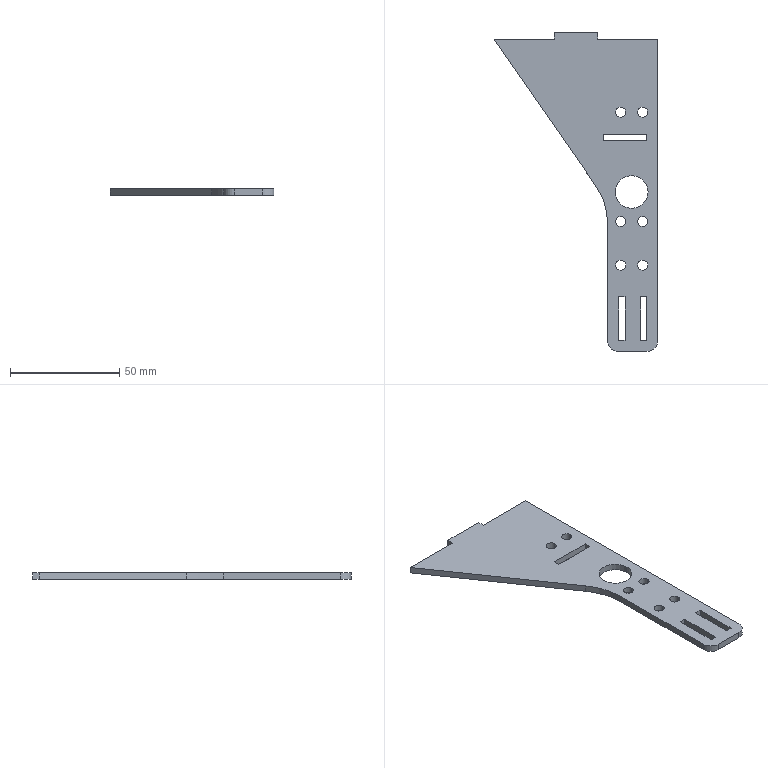Part | SolidWorks | features Cut 3, Fillet 2, Extrusion 1 | 1 solid | 40 faces | box 75 x 146 x 3 mm | volume 14540 mm3 | plane 23 | cylinder 17 | commonest cylinder face diameters 4.6 x12 10 x2 15 x2 60 x1
STEP:
#1=CARTESIAN_POINT('',(-9.25,39.5,0.));
#2=VERTEX_POINT('',#1);
#3=CARTESIAN_POINT('',(-4.65,39.5,0.));
#4=VERTEX_POINT('',#3);
#5=CARTESIAN_POINT('',(-6.95,39.5,0.));
#6=DIRECTION('',(0.,0.,1.));
#7=DIRECTION('',(1.,0.,0.));
#8=AXIS2_PLACEMENT_3D('',#5,#6,#7);
#9=CIRCLE('',#8,2.3);
#10=EDGE_CURVE('',#2,#4,#9,.T.);
#11=ORIENTED_EDGE('',*,*,#10,.F.);
#12=CARTESIAN_POINT('',(-9.25,39.5,3.));
#13=VERTEX_POINT('',#12);
#14=CARTESIAN_POINT('',(-9.25,39.5,0.));
#15=DIRECTION('',(0.,0.,1.));
#16=VECTOR('',#15,1000.);
#17=LINE('',#14,#16);
#18=EDGE_CURVE('',#2,#13,#17,.T.);
#19=ORIENTED_EDGE('',*,*,#18,.T.);
#20=CARTESIAN_POINT('',(-4.65,39.5,3.));
#21=VERTEX_POINT('',#20);
#22=CARTESIAN_POINT('',(-6.95,39.5,3.));
#23=DIRECTION('',(0.,0.,1.));
#24=DIRECTION('',(1.,0.,0.));
#25=AXIS2_PLACEMENT_3D('',#22,#23,#24);
#26=CIRCLE('',#25,2.3);
#27=EDGE_CURVE('',#13,#21,#26,.T.);
#28=ORIENTED_EDGE('',*,*,#27,.T.);
#29=CARTESIAN_POINT('',(-4.65,39.5,0.));
#30=DIRECTION('',(0.,0.,1.));
#31=VECTOR('',#30,1000.);
#32=LINE('',#29,#31);
#33=EDGE_CURVE('',#4,#21,#32,.T.);
#34=ORIENTED_EDGE('',*,*,#33,.F.);
#35=EDGE_LOOP('',(#11,#19,#28,#34));
#36=FACE_OUTER_BOUND('',#35,.T.);
#37=CARTESIAN_POINT('',(-6.95,39.5,0.));
#38=DIRECTION('',(0.,0.,1.));
#39=DIRECTION('',(1.,0.,0.));
#40=AXIS2_PLACEMENT_3D('',#37,#38,#39);
#41=CYLINDRICAL_SURFACE('',#40,2.3);
#42=ADVANCED_FACE('',(#36),#41,.F.);
#43=CARTESIAN_POINT('',(-19.35,39.5,0.));
#44=VERTEX_POINT('',#43);
#45=CARTESIAN_POINT('',(-14.75,39.5,0.));
#46=VERTEX_POINT('',#45);
#47=CARTESIAN_POINT('',(-17.05,39.5,0.));
#48=DIRECTION('',(0.,0.,1.));
#49=DIRECTION('',(1.,0.,0.));
#50=AXIS2_PLACEMENT_3D('',#47,#48,#49);
#51=CIRCLE('',#50,2.3);
#52=EDGE_CURVE('',#44,#46,#51,.T.);
#53=ORIENTED_EDGE('',*,*,#52,.F.);
#54=CARTESIAN_POINT('',(-19.35,39.5,3.));
#55=VERTEX_POINT('',#54);
#56=CARTESIAN_POINT('',(-19.35,39.5,0.));
#57=DIRECTION('',(0.,0.,1.));
#58=VECTOR('',#57,1000.);
#59=LINE('',#56,#58);
#60=EDGE_CURVE('',#44,#55,#59,.T.);
#61=ORIENTED_EDGE('',*,*,#60,.T.);
#62=CARTESIAN_POINT('',(-14.75,39.5,3.));
#63=VERTEX_POINT('',#62);
#64=CARTESIAN_POINT('',(-17.05,39.5,3.));
#65=DIRECTION('',(0.,0.,1.));
#66=DIRECTION('',(1.,0.,0.));
#67=AXIS2_PLACEMENT_3D('',#64,#65,#66);
#68=CIRCLE('',#67,2.3);
#69=EDGE_CURVE('',#55,#63,#68,.T.);
#70=ORIENTED_EDGE('',*,*,#69,.T.);
#71=CARTESIAN_POINT('',(-14.75,39.5,0.));
#72=DIRECTION('',(0.,0.,1.));
#73=VECTOR('',#72,1000.);
#74=LINE('',#71,#73);
#75=EDGE_CURVE('',#46,#63,#74,.T.);
#76=ORIENTED_EDGE('',*,*,#75,.F.);
#77=EDGE_LOOP('',(#53,#61,#70,#76));
#78=FACE_OUTER_BOUND('',#77,.T.);
#79=CARTESIAN_POINT('',(-17.05,39.5,0.));
#80=DIRECTION('',(0.,0.,1.));
#81=DIRECTION('',(1.,0.,0.));
#82=AXIS2_PLACEMENT_3D('',#79,#80,#81);
#83=CYLINDRICAL_SURFACE('',#82,2.3);
#84=ADVANCED_FACE('',(#78),#83,.F.);
#85=CARTESIAN_POINT('',(-4.65,109.5,3.));
#86=VERTEX_POINT('',#85);
#87=CARTESIAN_POINT('',(-9.25,109.5,3.));
#88=VERTEX_POINT('',#87);
#89=CARTESIAN_POINT('',(-6.95,109.5,3.));
#90=DIRECTION('',(0.,0.,-1.));
#91=DIRECTION('',(1.,0.,0.));
#92=AXIS2_PLACEMENT_3D('',#89,#90,#91);
#93=CIRCLE('',#92,2.3);
#94=EDGE_CURVE('',#86,#88,#93,.T.);
#95=ORIENTED_EDGE('',*,*,#94,.F.);
#96=CARTESIAN_POINT('',(-4.65,109.5,0.));
#97=VERTEX_POINT('',#96);
#98=CARTESIAN_POINT('',(-4.65,109.5,3.001));
#99=DIRECTION('',(0.,0.,-1.));
#100=VECTOR('',#99,1000.);
#101=LINE('',#98,#100);
#102=EDGE_CURVE('',#86,#97,#101,.T.);
#103=ORIENTED_EDGE('',*,*,#102,.T.);
#104=CARTESIAN_POINT('',(-9.25,109.5,0.));
#105=VERTEX_POINT('',#104);
#106=CARTESIAN_POINT('',(-6.95,109.5,0.));
#107=DIRECTION('',(0.,0.,-1.));
#108=DIRECTION('',(-1.,0.,0.));
#109=AXIS2_PLACEMENT_3D('',#106,#107,#108);
#110=CIRCLE('',#109,2.3);
#111=EDGE_CURVE('',#97,#105,#110,.T.);
#112=ORIENTED_EDGE('',*,*,#111,.T.);
#113=CARTESIAN_POINT('',(-9.25,109.5,3.001));
#114=DIRECTION('',(0.,0.,-1.));
#115=VECTOR('',#114,1000.);
#116=LINE('',#113,#115);
#117=EDGE_CURVE('',#88,#105,#116,.T.);
#118=ORIENTED_EDGE('',*,*,#117,.F.);
#119=EDGE_LOOP('',(#95,#103,#112,#118));
#120=FACE_OUTER_BOUND('',#119,.T.);
#121=CARTESIAN_POINT('',(-6.95,109.5,3.001));
#122=DIRECTION('',(0.,0.,-1.));
#123=DIRECTION('',(-1.,0.,0.));
#124=AXIS2_PLACEMENT_3D('',#121,#122,#123);
#125=CYLINDRICAL_SURFACE('',#124,2.3);
#126=ADVANCED_FACE('',(#120),#125,.F.);
#127=CARTESIAN_POINT('',(-14.75,109.5,3.));
#128=VERTEX_POINT('',#127);
#129=CARTESIAN_POINT('',(-19.35,109.5,3.));
#130=VERTEX_POINT('',#129);
#131=CARTESIAN_POINT('',(-17.05,109.5,3.));
#132=DIRECTION('',(0.,0.,-1.));
#133=DIRECTION('',(1.,0.,0.));
#134=AXIS2_PLACEMENT_3D('',#131,#132,#133);
#135=CIRCLE('',#134,2.3);
#136=EDGE_CURVE('',#128,#130,#135,.T.);
#137=ORIENTED_EDGE('',*,*,#136,.F.);
#138=CARTESIAN_POINT('',(-14.75,109.5,0.));
#139=VERTEX_POINT('',#138);
#140=CARTESIAN_POINT('',(-14.75,109.5,3.001));
#141=DIRECTION('',(0.,0.,-1.));
#142=VECTOR('',#141,1000.);
#143=LINE('',#140,#142);
#144=EDGE_CURVE('',#128,#139,#143,.T.);
#145=ORIENTED_EDGE('',*,*,#144,.T.);
#146=CARTESIAN_POINT('',(-19.35,109.5,0.));
#147=VERTEX_POINT('',#146);
#148=CARTESIAN_POINT('',(-17.05,109.5,0.));
#149=DIRECTION('',(0.,0.,-1.));
#150=DIRECTION('',(-1.,0.,0.));
#151=AXIS2_PLACEMENT_3D('',#148,#149,#150);
#152=CIRCLE('',#151,2.3);
#153=EDGE_CURVE('',#139,#147,#152,.T.);
#154=ORIENTED_EDGE('',*,*,#153,.T.);
#155=CARTESIAN_POINT('',(-19.35,109.5,3.001));
#156=DIRECTION('',(0.,0.,-1.));
#157=VECTOR('',#156,1000.);
#158=LINE('',#155,#157);
#159=EDGE_CURVE('',#130,#147,#158,.T.);
#160=ORIENTED_EDGE('',*,*,#159,.F.);
#161=EDGE_LOOP('',(#137,#145,#154,#160));
#162=FACE_OUTER_BOUND('',#161,.T.);
#163=CARTESIAN_POINT('',(-17.05,109.5,3.001));
#164=DIRECTION('',(0.,0.,-1.));
#165=DIRECTION('',(-1.,0.,0.));
#166=AXIS2_PLACEMENT_3D('',#163,#164,#165);
#167=CYLINDRICAL_SURFACE('',#166,2.3);
#168=ADVANCED_FACE('',(#162),#167,.F.);
#169=CARTESIAN_POINT('',(-4.65,59.5,3.));
#170=VERTEX_POINT('',#169);
#171=CARTESIAN_POINT('',(-9.25,59.5,3.));
#172=VERTEX_POINT('',#171);
#173=CARTESIAN_POINT('',(-6.95,59.5,3.));
#174=DIRECTION('',(0.,0.,-1.));
#175=DIRECTION('',(1.,0.,0.));
#176=AXIS2_PLACEMENT_3D('',#173,#174,#175);
#177=CIRCLE('',#176,2.3);
#178=EDGE_CURVE('',#170,#172,#177,.T.);
#179=ORIENTED_EDGE('',*,*,#178,.F.);
#180=CARTESIAN_POINT('',(-4.65,59.5,0.));
#181=VERTEX_POINT('',#180);
#182=CARTESIAN_POINT('',(-4.65,59.5,3.001));
#183=DIRECTION('',(0.,0.,-1.));
#184=VECTOR('',#183,1000.);
#185=LINE('',#182,#184);
#186=EDGE_CURVE('',#170,#181,#185,.T.);
#187=ORIENTED_EDGE('',*,*,#186,.T.);
#188=CARTESIAN_POINT('',(-9.25,59.5,0.));
#189=VERTEX_POINT('',#188);
#190=CARTESIAN_POINT('',(-6.95,59.5,0.));
#191=DIRECTION('',(0.,0.,-1.));
#192=DIRECTION('',(-1.,0.,0.));
#193=AXIS2_PLACEMENT_3D('',#190,#191,#192);
#194=CIRCLE('',#193,2.3);
#195=EDGE_CURVE('',#181,#189,#194,.T.);
#196=ORIENTED_EDGE('',*,*,#195,.T.);
#197=CARTESIAN_POINT('',(-9.25,59.5,3.001));
#198=DIRECTION('',(0.,0.,-1.));
#199=VECTOR('',#198,1000.);
#200=LINE('',#197,#199);
#201=EDGE_CURVE('',#172,#189,#200,.T.);
#202=ORIENTED_EDGE('',*,*,#201,.F.);
#203=EDGE_LOOP('',(#179,#187,#196,#202));
#204=FACE_OUTER_BOUND('',#203,.T.);
#205=CARTESIAN_POINT('',(-6.95,59.5,3.001));
#206=DIRECTION('',(0.,0.,-1.));
#207=DIRECTION('',(-1.,0.,0.));
#208=AXIS2_PLACEMENT_3D('',#205,#206,#207);
#209=CYLINDRICAL_SURFACE('',#208,2.3);
#210=ADVANCED_FACE('',(#204),#209,.F.);
#211=CARTESIAN_POINT('',(-14.75,59.5,3.));
#212=VERTEX_POINT('',#211);
#213=CARTESIAN_POINT('',(-19.35,59.5,3.));
#214=VERTEX_POINT('',#213);
#215=CARTESIAN_POINT('',(-17.05,59.5,3.));
#216=DIRECTION('',(0.,0.,-1.));
#217=DIRECTION('',(1.,0.,0.));
#218=AXIS2_PLACEMENT_3D('',#215,#216,#217);
#219=CIRCLE('',#218,2.3);
#220=EDGE_CURVE('',#212,#214,#219,.T.);
#221=ORIENTED_EDGE('',*,*,#220,.F.);
#222=CARTESIAN_POINT('',(-14.75,59.5,0.));
#223=VERTEX_POINT('',#222);
#224=CARTESIAN_POINT('',(-14.75,59.5,3.001));
#225=DIRECTION('',(0.,0.,-1.));
#226=VECTOR('',#225,1000.);
#227=LINE('',#224,#226);
#228=EDGE_CURVE('',#212,#223,#227,.T.);
#229=ORIENTED_EDGE('',*,*,#228,.T.);
#230=CARTESIAN_POINT('',(-19.35,59.5,0.));
#231=VERTEX_POINT('',#230);
#232=CARTESIAN_POINT('',(-17.05,59.5,0.));
#233=DIRECTION('',(0.,0.,-1.));
#234=DIRECTION('',(-1.,0.,0.));
#235=AXIS2_PLACEMENT_3D('',#232,#233,#234);
#236=CIRCLE('',#235,2.3);
#237=EDGE_CURVE('',#223,#231,#236,.T.);
#238=ORIENTED_EDGE('',*,*,#237,.T.);
#239=CARTESIAN_POINT('',(-19.35,59.5,3.001));
#240=DIRECTION('',(0.,0.,-1.));
#241=VECTOR('',#240,1000.);
#242=LINE('',#239,#241);
#243=EDGE_CURVE('',#214,#231,#242,.T.);
#244=ORIENTED_EDGE('',*,*,#243,.F.);
#245=EDGE_LOOP('',(#221,#229,#238,#244));
#246=FACE_OUTER_BOUND('',#245,.T.);
#247=CARTESIAN_POINT('',(-17.05,59.5,3.001));
#248=DIRECTION('',(0.,0.,-1.));
#249=DIRECTION('',(-1.,0.,0.));
#250=AXIS2_PLACEMENT_3D('',#247,#248,#249);
#251=CYLINDRICAL_SURFACE('',#250,2.3);
#252=ADVANCED_FACE('',(#246),#251,.F.);
#253=CARTESIAN_POINT('',(-4.5,73.,3.));
#254=VERTEX_POINT('',#253);
#255=CARTESIAN_POINT('',(-19.5,73.,3.));
#256=VERTEX_POINT('',#255);
#257=CARTESIAN_POINT('',(-12.,73.,3.));
#258=DIRECTION('',(0.,0.,-1.));
#259=DIRECTION('',(1.,0.,0.));
#260=AXIS2_PLACEMENT_3D('',#257,#258,#259);
#261=CIRCLE('',#260,7.5);
#262=EDGE_CURVE('',#254,#256,#261,.T.);
#263=ORIENTED_EDGE('',*,*,#262,.F.);
#264=CARTESIAN_POINT('',(-4.5,73.,0.));
#265=VERTEX_POINT('',#264);
#266=CARTESIAN_POINT('',(-4.5,73.,3.001));
#267=DIRECTION('',(0.,0.,-1.));
#268=VECTOR('',#267,1000.);
#269=LINE('',#266,#268);
#270=EDGE_CURVE('',#254,#265,#269,.T.);
#271=ORIENTED_EDGE('',*,*,#270,.T.);
#272=CARTESIAN_POINT('',(-19.5,73.,0.));
#273=VERTEX_POINT('',#272);
#274=CARTESIAN_POINT('',(-12.,73.,0.));
#275=DIRECTION('',(0.,0.,-1.));
#276=DIRECTION('',(-1.,0.,0.));
#277=AXIS2_PLACEMENT_3D('',#274,#275,#276);
#278=CIRCLE('',#277,7.5);
#279=EDGE_CURVE('',#265,#273,#278,.T.);
#280=ORIENTED_EDGE('',*,*,#279,.T.);
#281=CARTESIAN_POINT('',(-19.5,73.,3.001));
#282=DIRECTION('',(0.,0.,-1.));
#283=VECTOR('',#282,1000.);
#284=LINE('',#281,#283);
#285=EDGE_CURVE('',#256,#273,#284,.T.);
#286=ORIENTED_EDGE('',*,*,#285,.F.);
#287=EDGE_LOOP('',(#263,#271,#280,#286));
#288=FACE_OUTER_BOUND('',#287,.T.);
#289=CARTESIAN_POINT('',(-12.,73.,3.001));
#290=DIRECTION('',(0.,0.,-1.));
#291=DIRECTION('',(-1.,0.,0.));
#292=AXIS2_PLACEMENT_3D('',#289,#290,#291);
#293=CYLINDRICAL_SURFACE('',#292,7.5);
#294=ADVANCED_FACE('',(#288),#293,.F.);
#295=CARTESIAN_POINT('',(-6.95,39.5,3.));
#296=DIRECTION('',(0.,0.,1.));
#297=DIRECTION('',(1.,0.,0.));
#298=AXIS2_PLACEMENT_3D('',#295,#296,#297);
#299=CIRCLE('',#298,2.3);
#300=EDGE_CURVE('',#21,#13,#299,.T.);
#301=ORIENTED_EDGE('',*,*,#300,.F.);
#302=ORIENTED_EDGE('',*,*,#27,.F.);
#303=EDGE_LOOP('',(#301,#302));
#304=FACE_BOUND('',#303,.T.);
#305=CARTESIAN_POINT('',(-17.05,39.5,3.));
#306=DIRECTION('',(0.,0.,1.));
#307=DIRECTION('',(1.,0.,0.));
#308=AXIS2_PLACEMENT_3D('',#305,#306,#307);
#309=CIRCLE('',#308,2.3);
#310=EDGE_CURVE('',#63,#55,#309,.T.);
#311=ORIENTED_EDGE('',*,*,#310,.F.);
#312=ORIENTED_EDGE('',*,*,#69,.F.);
#313=EDGE_LOOP('',(#311,#312));
#314=FACE_BOUND('',#313,.T.);
#315=CARTESIAN_POINT('',(-5.,96.55,3.));
#316=VERTEX_POINT('',#315);
#317=CARTESIAN_POINT('',(-25.,96.55,3.));
#318=VERTEX_POINT('',#317);
#319=CARTESIAN_POINT('',(-5.,96.55,3.));
#320=DIRECTION('',(-1.,0.,0.));
#321=VECTOR('',#320,1000.);
#322=LINE('',#319,#321);
#323=EDGE_CURVE('',#316,#318,#322,.T.);
#324=ORIENTED_EDGE('',*,*,#323,.T.);
#325=CARTESIAN_POINT('',(-25.,99.45,3.));
#326=VERTEX_POINT('',#325);
#327=CARTESIAN_POINT('',(-25.,96.55,3.));
#328=DIRECTION('',(0.,1.,0.));
#329=VECTOR('',#328,1000.);
#330=LINE('',#327,#329);
#331=EDGE_CURVE('',#318,#326,#330,.T.);
#332=ORIENTED_EDGE('',*,*,#331,.T.);
#333=CARTESIAN_POINT('',(-5.,99.45,3.));
#334=VERTEX_POINT('',#333);
#335=CARTESIAN_POINT('',(-25.,99.45,3.));
#336=DIRECTION('',(1.,0.,0.));
#337=VECTOR('',#336,1000.);
#338=LINE('',#335,#337);
#339=EDGE_CURVE('',#326,#334,#338,.T.);
#340=ORIENTED_EDGE('',*,*,#339,.T.);
#341=CARTESIAN_POINT('',(-5.,99.45,3.));
#342=DIRECTION('',(0.,-1.,0.));
#343=VECTOR('',#342,1000.);
#344=LINE('',#341,#343);
#345=EDGE_CURVE('',#334,#316,#344,.T.);
#346=ORIENTED_EDGE('',*,*,#345,.T.);
#347=EDGE_LOOP('',(#324,#332,#340,#346));
#348=FACE_BOUND('',#347,.T.);
#349=CARTESIAN_POINT('',(-6.95,109.5,3.));
#350=DIRECTION('',(0.,0.,-1.));
#351=DIRECTION('',(1.,0.,0.));
#352=AXIS2_PLACEMENT_3D('',#349,#350,#351);
#353=CIRCLE('',#352,2.3);
#354=EDGE_CURVE('',#88,#86,#353,.T.);
#355=ORIENTED_EDGE('',*,*,#354,.T.);
#356=ORIENTED_EDGE('',*,*,#94,.T.);
#357=EDGE_LOOP('',(#355,#356));
#358=FACE_BOUND('',#357,.T.);
#359=CARTESIAN_POINT('',(-17.05,109.5,3.));
#360=DIRECTION('',(0.,0.,-1.));
#361=DIRECTION('',(1.,0.,0.));
#362=AXIS2_PLACEMENT_3D('',#359,#360,#361);
#363=CIRCLE('',#362,2.3);
#364=EDGE_CURVE('',#130,#128,#363,.T.);
#365=ORIENTED_EDGE('',*,*,#364,.T.);
#366=ORIENTED_EDGE('',*,*,#136,.T.);
#367=EDGE_LOOP('',(#365,#366));
#368=FACE_BOUND('',#367,.T.);
#369=CARTESIAN_POINT('',(-6.95,59.5,3.));
#370=DIRECTION('',(0.,0.,-1.));
#371=DIRECTION('',(1.,0.,0.));
#372=AXIS2_PLACEMENT_3D('',#369,#370,#371);
#373=CIRCLE('',#372,2.3);
#374=EDGE_CURVE('',#172,#170,#373,.T.);
#375=ORIENTED_EDGE('',*,*,#374,.T.);
#376=ORIENTED_EDGE('',*,*,#178,.T.);
#377=EDGE_LOOP('',(#375,#376));
#378=FACE_BOUND('',#377,.T.);
#379=CARTESIAN_POINT('',(-17.05,59.5,3.));
#380=DIRECTION('',(0.,0.,-1.));
#381=DIRECTION('',(1.,0.,0.));
#382=AXIS2_PLACEMENT_3D('',#379,#380,#381);
#383=CIRCLE('',#382,2.3);
#384=EDGE_CURVE('',#214,#212,#383,.T.);
#385=ORIENTED_EDGE('',*,*,#384,.T.);
#386=ORIENTED_EDGE('',*,*,#220,.T.);
#387=EDGE_LOOP('',(#385,#386));
#388=FACE_BOUND('',#387,.T.);
#389=CARTESIAN_POINT('',(-12.,73.,3.));
#390=DIRECTION('',(0.,0.,-1.));
#391=DIRECTION('',(1.,0.,0.));
#392=AXIS2_PLACEMENT_3D('',#389,#390,#391);
#393=CIRCLE('',#392,7.5);
#394=EDGE_CURVE('',#256,#254,#393,.T.);
#395=ORIENTED_EDGE('',*,*,#394,.T.);
#396=ORIENTED_EDGE('',*,*,#262,.T.);
#397=EDGE_LOOP('',(#395,#396));
#398=FACE_BOUND('',#397,.T.);
#399=CARTESIAN_POINT('',(-17.95,5.,3.));
#400=VERTEX_POINT('',#399);
#401=CARTESIAN_POINT('',(-15.05,5.,3.));
#402=VERTEX_POINT('',#401);
#403=CARTESIAN_POINT('',(-17.95,5.,3.));
#404=DIRECTION('',(1.,0.,0.));
#405=VECTOR('',#404,1000.);
#406=LINE('',#403,#405);
#407=EDGE_CURVE('',#400,#402,#406,.T.);
#408=ORIENTED_EDGE('',*,*,#407,.F.);
#409=CARTESIAN_POINT('',(-17.95,25.,3.));
#410=VERTEX_POINT('',#409);
#411=CARTESIAN_POINT('',(-17.95,25.,3.));
#412=DIRECTION('',(0.,-1.,0.));
#413=VECTOR('',#412,1000.);
#414=LINE('',#411,#413);
#415=EDGE_CURVE('',#410,#400,#414,.T.);
#416=ORIENTED_EDGE('',*,*,#415,.F.);
#417=CARTESIAN_POINT('',(-15.05,25.,3.));
#418=VERTEX_POINT('',#417);
#419=CARTESIAN_POINT('',(-17.95,25.,3.));
#420=DIRECTION('',(-1.,0.,0.));
#421=VECTOR('',#420,1000.);
#422=LINE('',#419,#421);
#423=EDGE_CURVE('',#418,#410,#422,.T.);
#424=ORIENTED_EDGE('',*,*,#423,.F.);
#425=CARTESIAN_POINT('',(-15.05,25.,3.));
#426=DIRECTION('',(0.,1.,0.));
#427=VECTOR('',#426,1000.);
#428=LINE('',#425,#427);
#429=EDGE_CURVE('',#402,#418,#428,.T.);
#430=ORIENTED_EDGE('',*,*,#429,.F.);
#431=EDGE_LOOP('',(#408,#416,#424,#430));
#432=FACE_BOUND('',#431,.T.);
#433=CARTESIAN_POINT('',(-18.,0.,3.));
#434=VERTEX_POINT('',#433);
#435=CARTESIAN_POINT('',(-5.,0.,3.));
#436=VERTEX_POINT('',#435);
#437=CARTESIAN_POINT('',(0.,0.,3.));
#438=DIRECTION('',(1.,0.,0.));
#439=VECTOR('',#438,1000.);
#440=LINE('',#437,#439);
#441=EDGE_CURVE('',#434,#436,#440,.T.);
#442=ORIENTED_EDGE('',*,*,#441,.T.);
#443=CARTESIAN_POINT('',(0.,5.,3.));
#444=VERTEX_POINT('',#443);
#445=CARTESIAN_POINT('',(-5.,5.,3.));
#446=DIRECTION('',(0.,0.,1.));
#447=DIRECTION('',(1.,0.,0.));
#448=AXIS2_PLACEMENT_3D('',#445,#446,#447);
#449=CIRCLE('',#448,5.);
#450=EDGE_CURVE('',#436,#444,#449,.T.);
#451=ORIENTED_EDGE('',*,*,#450,.T.);
#452=CARTESIAN_POINT('',(0.,143.,3.));
#453=VERTEX_POINT('',#452);
#454=CARTESIAN_POINT('',(0.,0.,3.));
#455=DIRECTION('',(0.,1.,0.));
#456=VECTOR('',#455,1000.);
#457=LINE('',#454,#456);
#458=EDGE_CURVE('',#444,#453,#457,.T.);
#459=ORIENTED_EDGE('',*,*,#458,.T.);
#460=CARTESIAN_POINT('',(-27.5,143.,3.));
#461=VERTEX_POINT('',#460);
#462=CARTESIAN_POINT('',(0.,143.,3.));
#463=DIRECTION('',(-1.,0.,0.));
#464=VECTOR('',#463,1000.);
#465=LINE('',#462,#464);
#466=EDGE_CURVE('',#453,#461,#465,.T.);
#467=ORIENTED_EDGE('',*,*,#466,.T.);
#468=CARTESIAN_POINT('',(-27.5,146.,3.));
#469=VERTEX_POINT('',#468);
#470=CARTESIAN_POINT('',(-27.5,143.,3.));
#471=DIRECTION('',(0.,1.,0.));
#472=VECTOR('',#471,1000.);
#473=LINE('',#470,#472);
#474=EDGE_CURVE('',#461,#469,#473,.T.);
#475=ORIENTED_EDGE('',*,*,#474,.T.);
#476=CARTESIAN_POINT('',(-47.5,146.,3.));
#477=VERTEX_POINT('',#476);
#478=CARTESIAN_POINT('',(-47.5,146.,3.));
#479=DIRECTION('',(-1.,0.,0.));
#480=VECTOR('',#479,1000.);
#481=LINE('',#478,#480);
#482=EDGE_CURVE('',#469,#477,#481,.T.);
#483=ORIENTED_EDGE('',*,*,#482,.T.);
#484=CARTESIAN_POINT('',(-47.5,143.,3.));
#485=VERTEX_POINT('',#484);
#486=CARTESIAN_POINT('',(-47.5,143.,3.));
#487=DIRECTION('',(0.,-1.,0.));
#488=VECTOR('',#487,1000.);
#489=LINE('',#486,#488);
#490=EDGE_CURVE('',#477,#485,#489,.T.);
#491=ORIENTED_EDGE('',*,*,#490,.T.);
#492=CARTESIAN_POINT('',(-75.,143.,3.));
#493=VERTEX_POINT('',#492);
#494=CARTESIAN_POINT('',(-75.,143.,3.));
#495=DIRECTION('',(-1.,0.,0.));
#496=VECTOR('',#495,1000.);
#497=LINE('',#494,#496);
#498=EDGE_CURVE('',#485,#493,#497,.T.);
#499=ORIENTED_EDGE('',*,*,#498,.T.);
#500=CARTESIAN_POINT('',(-28.346,75.711,3.));
#501=VERTEX_POINT('',#500);
#502=CARTESIAN_POINT('',(-23.,68.,3.));
#503=DIRECTION('',(0.5698,-0.8218,0.));
#504=VECTOR('',#503,1000.);
#505=LINE('',#502,#504);
#506=EDGE_CURVE('',#493,#501,#505,.T.);
#507=ORIENTED_EDGE('',*,*,#506,.T.);
#508=CARTESIAN_POINT('',(-23.,58.617,3.));
#509=VERTEX_POINT('',#508);
#510=CARTESIAN_POINT('',(-53.,58.617,3.));
#511=DIRECTION('',(0.,0.,-1.));
#512=DIRECTION('',(1.,0.,0.));
#513=AXIS2_PLACEMENT_3D('',#510,#511,#512);
#514=CIRCLE('',#513,30.);
#515=EDGE_CURVE('',#501,#509,#514,.T.);
#516=ORIENTED_EDGE('',*,*,#515,.T.);
#517=CARTESIAN_POINT('',(-23.,5.,3.));
#518=VERTEX_POINT('',#517);
#519=CARTESIAN_POINT('',(-23.,0.,3.));
#520=DIRECTION('',(0.,-1.,0.));
#521=VECTOR('',#520,1000.);
#522=LINE('',#519,#521);
#523=EDGE_CURVE('',#509,#518,#522,.T.);
#524=ORIENTED_EDGE('',*,*,#523,.T.);
#525=CARTESIAN_POINT('',(-18.,5.,3.));
#526=DIRECTION('',(0.,0.,1.));
#527=DIRECTION('',(1.,0.,0.));
#528=AXIS2_PLACEMENT_3D('',#525,#526,#527);
#529=CIRCLE('',#528,5.);
#530=EDGE_CURVE('',#518,#434,#529,.T.);
#531=ORIENTED_EDGE('',*,*,#530,.T.);
#532=EDGE_LOOP('',(#442,#451,#459,#467,#475,#483,#491,#499,#507,#516,#524,#531));
#533=FACE_OUTER_BOUND('',#532,.T.);
#534=CARTESIAN_POINT('',(-7.95,5.,3.));
#535=VERTEX_POINT('',#534);
#536=CARTESIAN_POINT('',(-5.05,5.,3.));
#537=VERTEX_POINT('',#536);
#538=CARTESIAN_POINT('',(-7.95,5.,3.));
#539=DIRECTION('',(1.,0.,0.));
#540=VECTOR('',#539,1000.);
#541=LINE('',#538,#540);
#542=EDGE_CURVE('',#535,#537,#541,.T.);
#543=ORIENTED_EDGE('',*,*,#542,.F.);
#544=CARTESIAN_POINT('',(-7.95,25.,3.));
#545=VERTEX_POINT('',#544);
#546=CARTESIAN_POINT('',(-7.95,5.,3.));
#547=DIRECTION('',(0.,-1.,0.));
#548=VECTOR('',#547,1000.);
#549=LINE('',#546,#548);
#550=EDGE_CURVE('',#545,#535,#549,.T.);
#551=ORIENTED_EDGE('',*,*,#550,.F.);
#552=CARTESIAN_POINT('',(-5.05,25.,3.));
#553=VERTEX_POINT('',#552);
#554=CARTESIAN_POINT('',(-7.95,25.,3.));
#555=DIRECTION('',(-1.,0.,0.));
#556=VECTOR('',#555,1000.);
#557=LINE('',#554,#556);
#558=EDGE_CURVE('',#553,#545,#557,.T.);
#559=ORIENTED_EDGE('',*,*,#558,.F.);
#560=CARTESIAN_POINT('',(-5.05,5.,3.));
#561=DIRECTION('',(0.,1.,0.));
#562=VECTOR('',#561,1000.);
#563=LINE('',#560,#562);
#564=EDGE_CURVE('',#537,#553,#563,.T.);
#565=ORIENTED_EDGE('',*,*,#564,.F.);
#566=EDGE_LOOP('',(#543,#551,#559,#565));
#567=FACE_BOUND('',#566,.T.);
#568=CARTESIAN_POINT('',(0.,0.,3.));
#569=DIRECTION('',(0.,0.,1.));
#570=DIRECTION('',(1.,0.,0.));
#571=AXIS2_PLACEMENT_3D('',#568,#569,#570);
#572=PLANE('',#571);
#573=ADVANCED_FACE('',(#304,#314,#348,#358,#368,#378,#388,#398,#432,#533,#567),#572,.T.);
#574=CARTESIAN_POINT('',(-6.95,39.5,0.));
#575=DIRECTION('',(0.,0.,1.));
#576=DIRECTION('',(1.,0.,0.));
#577=AXIS2_PLACEMENT_3D('',#574,#575,#576);
#578=CIRCLE('',#577,2.3);
#579=EDGE_CURVE('',#4,#2,#578,.T.);
#580=ORIENTED_EDGE('',*,*,#579,.T.);
#581=ORIENTED_EDGE('',*,*,#10,.T.);
#582=EDGE_LOOP('',(#580,#581));
#583=FACE_BOUND('',#582,.T.);
#584=CARTESIAN_POINT('',(-17.05,39.5,0.));
#585=DIRECTION('',(0.,0.,1.));
#586=DIRECTION('',(1.,0.,0.));
#587=AXIS2_PLACEMENT_3D('',#584,#585,#586);
#588=CIRCLE('',#587,2.3);
#589=EDGE_CURVE('',#46,#44,#588,.T.);
#590=ORIENTED_EDGE('',*,*,#589,.T.);
#591=ORIENTED_EDGE('',*,*,#52,.T.);
#592=EDGE_LOOP('',(#590,#591));
#593=FACE_BOUND('',#592,.T.);
#594=CARTESIAN_POINT('',(-25.,96.55,0.));
#595=VERTEX_POINT('',#594);
#596=CARTESIAN_POINT('',(-25.,99.45,0.));
#597=VERTEX_POINT('',#596);
#598=CARTESIAN_POINT('',(-25.,96.55,0.));
#599=DIRECTION('',(0.,1.,0.));
#600=VECTOR('',#599,1000.);
#601=LINE('',#598,#600);
#602=EDGE_CURVE('',#595,#597,#601,.T.);
#603=ORIENTED_EDGE('',*,*,#602,.F.);
#604=CARTESIAN_POINT('',(-5.,96.55,0.));
#605=VERTEX_POINT('',#604);
#606=CARTESIAN_POINT('',(-5.,96.55,0.));
#607=DIRECTION('',(-1.,0.,0.));
#608=VECTOR('',#607,1000.);
#609=LINE('',#606,#608);
#610=EDGE_CURVE('',#605,#595,#609,.T.);
#611=ORIENTED_EDGE('',*,*,#610,.F.);
#612=CARTESIAN_POINT('',(-5.,99.45,0.));
#613=VERTEX_POINT('',#612);
#614=CARTESIAN_POINT('',(-5.,99.45,0.));
#615=DIRECTION('',(0.,-1.,0.));
#616=VECTOR('',#615,1000.);
#617=LINE('',#614,#616);
#618=EDGE_CURVE('',#613,#605,#617,.T.);
#619=ORIENTED_EDGE('',*,*,#618,.F.);
#620=CARTESIAN_POINT('',(-25.,99.45,0.));
#621=DIRECTION('',(1.,0.,0.));
#622=VECTOR('',#621,1000.);
#623=LINE('',#620,#622);
#624=EDGE_CURVE('',#597,#613,#623,.T.);
#625=ORIENTED_EDGE('',*,*,#624,.F.);
#626=EDGE_LOOP('',(#603,#611,#619,#625));
#627=FACE_BOUND('',#626,.T.);
#628=CARTESIAN_POINT('',(-6.95,109.5,0.));
#629=DIRECTION('',(0.,0.,-1.));
#630=DIRECTION('',(-1.,0.,0.));
#631=AXIS2_PLACEMENT_3D('',#628,#629,#630);
#632=CIRCLE('',#631,2.3);
#633=EDGE_CURVE('',#105,#97,#632,.T.);
#634=ORIENTED_EDGE('',*,*,#633,.F.);
#635=ORIENTED_EDGE('',*,*,#111,.F.);
#636=EDGE_LOOP('',(#634,#635));
#637=FACE_BOUND('',#636,.T.);
#638=CARTESIAN_POINT('',(-17.05,109.5,0.));
#639=DIRECTION('',(0.,0.,-1.));
#640=DIRECTION('',(-1.,0.,0.));
#641=AXIS2_PLACEMENT_3D('',#638,#639,#640);
#642=CIRCLE('',#641,2.3);
#643=EDGE_CURVE('',#147,#139,#642,.T.);
#644=ORIENTED_EDGE('',*,*,#643,.F.);
#645=ORIENTED_EDGE('',*,*,#153,.F.);
#646=EDGE_LOOP('',(#644,#645));
#647=FACE_BOUND('',#646,.T.);
#648=CARTESIAN_POINT('',(-6.95,59.5,0.));
#649=DIRECTION('',(0.,0.,-1.));
#650=DIRECTION('',(-1.,0.,0.));
#651=AXIS2_PLACEMENT_3D('',#648,#649,#650);
#652=CIRCLE('',#651,2.3);
#653=EDGE_CURVE('',#189,#181,#652,.T.);
#654=ORIENTED_EDGE('',*,*,#653,.F.);
#655=ORIENTED_EDGE('',*,*,#195,.F.);
#656=EDGE_LOOP('',(#654,#655));
#657=FACE_BOUND('',#656,.T.);
#658=CARTESIAN_POINT('',(-17.05,59.5,0.));
#659=DIRECTION('',(0.,0.,-1.));
#660=DIRECTION('',(-1.,0.,0.));
#661=AXIS2_PLACEMENT_3D('',#658,#659,#660);
#662=CIRCLE('',#661,2.3);
#663=EDGE_CURVE('',#231,#223,#662,.T.);
#664=ORIENTED_EDGE('',*,*,#663,.F.);
#665=ORIENTED_EDGE('',*,*,#237,.F.);
#666=EDGE_LOOP('',(#664,#665));
#667=FACE_BOUND('',#666,.T.);
#668=CARTESIAN_POINT('',(-12.,73.,0.));
#669=DIRECTION('',(0.,0.,-1.));
#670=DIRECTION('',(-1.,0.,0.));
#671=AXIS2_PLACEMENT_3D('',#668,#669,#670);
#672=CIRCLE('',#671,7.5);
#673=EDGE_CURVE('',#273,#265,#672,.T.);
#674=ORIENTED_EDGE('',*,*,#673,.F.);
#675=ORIENTED_EDGE('',*,*,#279,.F.);
#676=EDGE_LOOP('',(#674,#675));
#677=FACE_BOUND('',#676,.T.);
#678=CARTESIAN_POINT('',(-17.95,25.,0.));
#679=VERTEX_POINT('',#678);
#680=CARTESIAN_POINT('',(-17.95,5.,0.));
#681=VERTEX_POINT('',#680);
#682=CARTESIAN_POINT('',(-17.95,25.,0.));
#683=DIRECTION('',(0.,-1.,0.));
#684=VECTOR('',#683,1000.);
#685=LINE('',#682,#684);
#686=EDGE_CURVE('',#679,#681,#685,.T.);
#687=ORIENTED_EDGE('',*,*,#686,.T.);
#688=CARTESIAN_POINT('',(-15.05,5.,0.));
#689=VERTEX_POINT('',#688);
#690=CARTESIAN_POINT('',(-17.95,5.,0.));
#691=DIRECTION('',(1.,0.,0.));
#692=VECTOR('',#691,1000.);
#693=LINE('',#690,#692);
#694=EDGE_CURVE('',#681,#689,#693,.T.);
#695=ORIENTED_EDGE('',*,*,#694,.T.);
#696=CARTESIAN_POINT('',(-15.05,25.,0.));
#697=VERTEX_POINT('',#696);
#698=CARTESIAN_POINT('',(-15.05,25.,0.));
#699=DIRECTION('',(0.,1.,0.));
#700=VECTOR('',#699,1000.);
#701=LINE('',#698,#700);
#702=EDGE_CURVE('',#689,#697,#701,.T.);
#703=ORIENTED_EDGE('',*,*,#702,.T.);
#704=CARTESIAN_POINT('',(-17.95,25.,0.));
#705=DIRECTION('',(-1.,0.,0.));
#706=VECTOR('',#705,1000.);
#707=LINE('',#704,#706);
#708=EDGE_CURVE('',#697,#679,#707,.T.);
#709=ORIENTED_EDGE('',*,*,#708,.T.);
#710=EDGE_LOOP('',(#687,#695,#703,#709));
#711=FACE_BOUND('',#710,.T.);
#712=CARTESIAN_POINT('',(0.,5.,0.));
#713=VERTEX_POINT('',#712);
#714=CARTESIAN_POINT('',(0.,143.,0.));
#715=VERTEX_POINT('',#714);
#716=CARTESIAN_POINT('',(0.,0.,0.));
#717=DIRECTION('',(0.,1.,0.));
#718=VECTOR('',#717,1000.);
#719=LINE('',#716,#718);
#720=EDGE_CURVE('',#713,#715,#719,.T.);
#721=ORIENTED_EDGE('',*,*,#720,.F.);
#722=CARTESIAN_POINT('',(-5.,0.,0.));
#723=VERTEX_POINT('',#722);
#724=CARTESIAN_POINT('',(-5.,5.,0.));
#725=DIRECTION('',(0.,0.,-1.));
#726=DIRECTION('',(1.,0.,0.));
#727=AXIS2_PLACEMENT_3D('',#724,#725,#726);
#728=CIRCLE('',#727,5.);
#729=EDGE_CURVE('',#713,#723,#728,.T.);
#730=ORIENTED_EDGE('',*,*,#729,.T.);
#731=CARTESIAN_POINT('',(-18.,0.,0.));
#732=VERTEX_POINT('',#731);
#733=CARTESIAN_POINT('',(0.,0.,0.));
#734=DIRECTION('',(1.,0.,0.));
#735=VECTOR('',#734,1000.);
#736=LINE('',#733,#735);
#737=EDGE_CURVE('',#732,#723,#736,.T.);
#738=ORIENTED_EDGE('',*,*,#737,.F.);
#739=CARTESIAN_POINT('',(-23.,5.,0.));
#740=VERTEX_POINT('',#739);
#741=CARTESIAN_POINT('',(-18.,5.,0.));
#742=DIRECTION('',(0.,0.,-1.));
#743=DIRECTION('',(1.,0.,0.));
#744=AXIS2_PLACEMENT_3D('',#741,#742,#743);
#745=CIRCLE('',#744,5.);
#746=EDGE_CURVE('',#732,#740,#745,.T.);
#747=ORIENTED_EDGE('',*,*,#746,.T.);
#748=CARTESIAN_POINT('',(-23.,58.617,0.));
#749=VERTEX_POINT('',#748);
#750=CARTESIAN_POINT('',(-23.,0.,0.));
#751=DIRECTION('',(0.,-1.,0.));
#752=VECTOR('',#751,1000.);
#753=LINE('',#750,#752);
#754=EDGE_CURVE('',#749,#740,#753,.T.);
#755=ORIENTED_EDGE('',*,*,#754,.F.);
#756=CARTESIAN_POINT('',(-28.346,75.711,0.));
#757=VERTEX_POINT('',#756);
#758=CARTESIAN_POINT('',(-53.,58.617,0.));
#759=DIRECTION('',(0.,0.,1.));
#760=DIRECTION('',(1.,0.,0.));
#761=AXIS2_PLACEMENT_3D('',#758,#759,#760);
#762=CIRCLE('',#761,30.);
#763=EDGE_CURVE('',#749,#757,#762,.T.);
#764=ORIENTED_EDGE('',*,*,#763,.T.);
#765=CARTESIAN_POINT('',(-75.,143.,0.));
#766=VERTEX_POINT('',#765);
#767=CARTESIAN_POINT('',(-23.,68.,0.));
#768=DIRECTION('',(0.5698,-0.8218,0.));
#769=VECTOR('',#768,1000.);
#770=LINE('',#767,#769);
#771=EDGE_CURVE('',#766,#757,#770,.T.);
#772=ORIENTED_EDGE('',*,*,#771,.F.);
#773=CARTESIAN_POINT('',(-47.5,143.,0.));
#774=VERTEX_POINT('',#773);
#775=CARTESIAN_POINT('',(-75.,143.,0.));
#776=DIRECTION('',(-1.,0.,0.));
#777=VECTOR('',#776,1000.);
#778=LINE('',#775,#777);
#779=EDGE_CURVE('',#774,#766,#778,.T.);
#780=ORIENTED_EDGE('',*,*,#779,.F.);
#781=CARTESIAN_POINT('',(-47.5,146.,0.));
#782=VERTEX_POINT('',#781);
#783=CARTESIAN_POINT('',(-47.5,143.,0.));
#784=DIRECTION('',(0.,-1.,0.));
#785=VECTOR('',#784,1000.);
#786=LINE('',#783,#785);
#787=EDGE_CURVE('',#782,#774,#786,.T.);
#788=ORIENTED_EDGE('',*,*,#787,.F.);
#789=CARTESIAN_POINT('',(-27.5,146.,0.));
#790=VERTEX_POINT('',#789);
#791=CARTESIAN_POINT('',(-47.5,146.,0.));
#792=DIRECTION('',(-1.,0.,0.));
#793=VECTOR('',#792,1000.);
#794=LINE('',#791,#793);
#795=EDGE_CURVE('',#790,#782,#794,.T.);
#796=ORIENTED_EDGE('',*,*,#795,.F.);
#797=CARTESIAN_POINT('',(-27.5,143.,0.));
#798=VERTEX_POINT('',#797);
#799=CARTESIAN_POINT('',(-27.5,143.,0.));
#800=DIRECTION('',(0.,1.,0.));
#801=VECTOR('',#800,1000.);
#802=LINE('',#799,#801);
#803=EDGE_CURVE('',#798,#790,#802,.T.);
#804=ORIENTED_EDGE('',*,*,#803,.F.);
#805=CARTESIAN_POINT('',(0.,143.,0.));
#806=DIRECTION('',(-1.,0.,0.));
#807=VECTOR('',#806,1000.);
#808=LINE('',#805,#807);
#809=EDGE_CURVE('',#715,#798,#808,.T.);
#810=ORIENTED_EDGE('',*,*,#809,.F.);
#811=EDGE_LOOP('',(#721,#730,#738,#747,#755,#764,#772,#780,#788,#796,#804,#810));
#812=FACE_OUTER_BOUND('',#811,.T.);
#813=CARTESIAN_POINT('',(-7.95,25.,0.));
#814=VERTEX_POINT('',#813);
#815=CARTESIAN_POINT('',(-7.95,5.,0.));
#816=VERTEX_POINT('',#815);
#817=CARTESIAN_POINT('',(-7.95,5.,0.));
#818=DIRECTION('',(0.,-1.,0.));
#819=VECTOR('',#818,1000.);
#820=LINE('',#817,#819);
#821=EDGE_CURVE('',#814,#816,#820,.T.);
#822=ORIENTED_EDGE('',*,*,#821,.T.);
#823=CARTESIAN_POINT('',(-5.05,5.,0.));
#824=VERTEX_POINT('',#823);
#825=CARTESIAN_POINT('',(-7.95,5.,0.));
#826=DIRECTION('',(1.,0.,0.));
#827=VECTOR('',#826,1000.);
#828=LINE('',#825,#827);
#829=EDGE_CURVE('',#816,#824,#828,.T.);
#830=ORIENTED_EDGE('',*,*,#829,.T.);
#831=CARTESIAN_POINT('',(-5.05,25.,0.));
#832=VERTEX_POINT('',#831);
#833=CARTESIAN_POINT('',(-5.05,5.,0.));
#834=DIRECTION('',(0.,1.,0.));
#835=VECTOR('',#834,1000.);
#836=LINE('',#833,#835);
#837=EDGE_CURVE('',#824,#832,#836,.T.);
#838=ORIENTED_EDGE('',*,*,#837,.T.);
#839=CARTESIAN_POINT('',(-7.95,25.,0.));
#840=DIRECTION('',(-1.,0.,0.));
#841=VECTOR('',#840,1000.);
#842=LINE('',#839,#841);
#843=EDGE_CURVE('',#832,#814,#842,.T.);
#844=ORIENTED_EDGE('',*,*,#843,.T.);
#845=EDGE_LOOP('',(#822,#830,#838,#844));
#846=FACE_BOUND('',#845,.T.);
#847=CARTESIAN_POINT('',(0.,0.,0.));
#848=DIRECTION('',(0.,0.,1.));
#849=DIRECTION('',(1.,0.,0.));
#850=AXIS2_PLACEMENT_3D('',#847,#848,#849);
#851=PLANE('',#850);
#852=ADVANCED_FACE('',(#583,#593,#627,#637,#647,#657,#667,#677,#711,#812,#846),#851,.F.);
#853=ORIENTED_EDGE('',*,*,#458,.F.);
#854=CARTESIAN_POINT('',(0.,5.,3.));
#855=DIRECTION('',(0.,0.,-1.));
#856=VECTOR('',#855,1000.);
#857=LINE('',#854,#856);
#858=EDGE_CURVE('',#444,#713,#857,.T.);
#859=ORIENTED_EDGE('',*,*,#858,.T.);
#860=ORIENTED_EDGE('',*,*,#720,.T.);
#861=CARTESIAN_POINT('',(0.,143.,3.));
#862=DIRECTION('',(0.,0.,-1.));
#863=VECTOR('',#862,1000.);
#864=LINE('',#861,#863);
#865=EDGE_CURVE('',#453,#715,#864,.T.);
#866=ORIENTED_EDGE('',*,*,#865,.F.);
#867=EDGE_LOOP('',(#853,#859,#860,#866));
#868=FACE_OUTER_BOUND('',#867,.T.);
#869=CARTESIAN_POINT('',(0.,0.,3.));
#870=DIRECTION('',(-1.,0.,0.));
#871=DIRECTION('',(0.,0.,1.));
#872=AXIS2_PLACEMENT_3D('',#869,#870,#871);
#873=PLANE('',#872);
#874=ADVANCED_FACE('',(#868),#873,.F.);
#875=ORIENTED_EDGE('',*,*,#809,.T.);
#876=CARTESIAN_POINT('',(-27.5,143.,3.));
#877=DIRECTION('',(0.,0.,-1.));
#878=VECTOR('',#877,1000.);
#879=LINE('',#876,#878);
#880=EDGE_CURVE('',#461,#798,#879,.T.);
#881=ORIENTED_EDGE('',*,*,#880,.F.);
#882=ORIENTED_EDGE('',*,*,#466,.F.);
#883=ORIENTED_EDGE('',*,*,#865,.T.);
#884=EDGE_LOOP('',(#875,#881,#882,#883));
#885=FACE_OUTER_BOUND('',#884,.T.);
#886=CARTESIAN_POINT('',(0.,143.,3.));
#887=DIRECTION('',(0.,-1.,0.));
#888=DIRECTION('',(0.,0.,-1.));
#889=AXIS2_PLACEMENT_3D('',#886,#887,#888);
#890=PLANE('',#889);
#891=ADVANCED_FACE('',(#885),#890,.F.);
#892=ORIENTED_EDGE('',*,*,#803,.T.);
#893=CARTESIAN_POINT('',(-27.5,146.,3.));
#894=DIRECTION('',(0.,0.,-1.));
#895=VECTOR('',#894,1000.);
#896=LINE('',#893,#895);
#897=EDGE_CURVE('',#469,#790,#896,.T.);
#898=ORIENTED_EDGE('',*,*,#897,.F.);
#899=ORIENTED_EDGE('',*,*,#474,.F.);
#900=ORIENTED_EDGE('',*,*,#880,.T.);
#901=EDGE_LOOP('',(#892,#898,#899,#900));
#902=FACE_OUTER_BOUND('',#901,.T.);
#903=CARTESIAN_POINT('',(-27.5,143.,3.));
#904=DIRECTION('',(-1.,0.,0.));
#905=DIRECTION('',(0.,0.,1.));
#906=AXIS2_PLACEMENT_3D('',#903,#904,#905);
#907=PLANE('',#906);
#908=ADVANCED_FACE('',(#902),#907,.F.);
#909=ORIENTED_EDGE('',*,*,#795,.T.);
#910=CARTESIAN_POINT('',(-47.5,146.,3.));
#911=DIRECTION('',(0.,0.,-1.));
#912=VECTOR('',#911,1000.);
#913=LINE('',#910,#912);
#914=EDGE_CURVE('',#477,#782,#913,.T.);
#915=ORIENTED_EDGE('',*,*,#914,.F.);
#916=ORIENTED_EDGE('',*,*,#482,.F.);
#917=ORIENTED_EDGE('',*,*,#897,.T.);
#918=EDGE_LOOP('',(#909,#915,#916,#917));
#919=FACE_OUTER_BOUND('',#918,.T.);
#920=CARTESIAN_POINT('',(-47.5,146.,3.));
#921=DIRECTION('',(0.,-1.,0.));
#922=DIRECTION('',(0.,0.,-1.));
#923=AXIS2_PLACEMENT_3D('',#920,#921,#922);
#924=PLANE('',#923);
#925=ADVANCED_FACE('',(#919),#924,.F.);
#926=ORIENTED_EDGE('',*,*,#787,.T.);
#927=CARTESIAN_POINT('',(-47.5,143.,3.));
#928=DIRECTION('',(0.,0.,-1.));
#929=VECTOR('',#928,1000.);
#930=LINE('',#927,#929);
#931=EDGE_CURVE('',#485,#774,#930,.T.);
#932=ORIENTED_EDGE('',*,*,#931,.F.);
#933=ORIENTED_EDGE('',*,*,#490,.F.);
#934=ORIENTED_EDGE('',*,*,#914,.T.);
#935=EDGE_LOOP('',(#926,#932,#933,#934));
#936=FACE_OUTER_BOUND('',#935,.T.);
#937=CARTESIAN_POINT('',(-47.5,143.,3.));
#938=DIRECTION('',(1.,0.,0.));
#939=DIRECTION('',(0.,0.,-1.));
#940=AXIS2_PLACEMENT_3D('',#937,#938,#939);
#941=PLANE('',#940);
#942=ADVANCED_FACE('',(#936),#941,.F.);
#943=ORIENTED_EDGE('',*,*,#779,.T.);
#944=CARTESIAN_POINT('',(-75.,143.,3.));
#945=DIRECTION('',(0.,0.,-1.));
#946=VECTOR('',#945,1000.);
#947=LINE('',#944,#946);
#948=EDGE_CURVE('',#493,#766,#947,.T.);
#949=ORIENTED_EDGE('',*,*,#948,.F.);
#950=ORIENTED_EDGE('',*,*,#498,.F.);
#951=ORIENTED_EDGE('',*,*,#931,.T.);
#952=EDGE_LOOP('',(#943,#949,#950,#951));
#953=FACE_OUTER_BOUND('',#952,.T.);
#954=CARTESIAN_POINT('',(-75.,143.,3.));
#955=DIRECTION('',(0.,-1.,0.));
#956=DIRECTION('',(0.,0.,-1.));
#957=AXIS2_PLACEMENT_3D('',#954,#955,#956);
#958=PLANE('',#957);
#959=ADVANCED_FACE('',(#953),#958,.F.);
#960=ORIENTED_EDGE('',*,*,#771,.T.);
#961=CARTESIAN_POINT('',(-28.346,75.711,3.));
#962=DIRECTION('',(0.,0.,1.));
#963=VECTOR('',#962,1000.);
#964=LINE('',#961,#963);
#965=EDGE_CURVE('',#757,#501,#964,.T.);
#966=ORIENTED_EDGE('',*,*,#965,.T.);
#967=ORIENTED_EDGE('',*,*,#506,.F.);
#968=ORIENTED_EDGE('',*,*,#948,.T.);
#969=EDGE_LOOP('',(#960,#966,#967,#968));
#970=FACE_OUTER_BOUND('',#969,.T.);
#971=CARTESIAN_POINT('',(-23.,68.,3.));
#972=DIRECTION('',(0.8218,0.5698,0.));
#973=DIRECTION('',(-0.5698,0.8218,0.));
#974=AXIS2_PLACEMENT_3D('',#971,#972,#973);
#975=PLANE('',#974);
#976=ADVANCED_FACE('',(#970),#975,.F.);
#977=ORIENTED_EDGE('',*,*,#523,.F.);
#978=CARTESIAN_POINT('',(-23.,58.617,0.));
#979=DIRECTION('',(0.,0.,-1.));
#980=VECTOR('',#979,1000.);
#981=LINE('',#978,#980);
#982=EDGE_CURVE('',#509,#749,#981,.T.);
#983=ORIENTED_EDGE('',*,*,#982,.T.);
#984=ORIENTED_EDGE('',*,*,#754,.T.);
#985=CARTESIAN_POINT('',(-23.,5.,3.));
#986=DIRECTION('',(0.,0.,1.));
#987=VECTOR('',#986,1000.);
#988=LINE('',#985,#987);
#989=EDGE_CURVE('',#740,#518,#988,.T.);
#990=ORIENTED_EDGE('',*,*,#989,.T.);
#991=EDGE_LOOP('',(#977,#983,#984,#990));
#992=FACE_OUTER_BOUND('',#991,.T.);
#993=CARTESIAN_POINT('',(-23.,0.,3.));
#994=DIRECTION('',(1.,0.,0.));
#995=DIRECTION('',(0.,0.,-1.));
#996=AXIS2_PLACEMENT_3D('',#993,#994,#995);
#997=PLANE('',#996);
#998=ADVANCED_FACE('',(#992),#997,.F.);
#999=ORIENTED_EDGE('',*,*,#737,.T.);
#1000=CARTESIAN_POINT('',(-5.,0.,3.));
#1001=DIRECTION('',(0.,0.,1.));
#1002=VECTOR('',#1001,1000.);
#1003=LINE('',#1000,#1002);
#1004=EDGE_CURVE('',#723,#436,#1003,.T.);
#1005=ORIENTED_EDGE('',*,*,#1004,.T.);
#1006=ORIENTED_EDGE('',*,*,#441,.F.);
#1007=CARTESIAN_POINT('',(-18.,0.,3.));
#1008=DIRECTION('',(0.,0.,-1.));
#1009=VECTOR('',#1008,1000.);
#1010=LINE('',#1007,#1009);
#1011=EDGE_CURVE('',#434,#732,#1010,.T.);
#1012=ORIENTED_EDGE('',*,*,#1011,.T.);
#1013=EDGE_LOOP('',(#999,#1005,#1006,#1012));
#1014=FACE_OUTER_BOUND('',#1013,.T.);
#1015=CARTESIAN_POINT('',(0.,0.,3.));
#1016=DIRECTION('',(0.,1.,0.));
#1017=DIRECTION('',(0.,0.,1.));
#1018=AXIS2_PLACEMENT_3D('',#1015,#1016,#1017);
#1019=PLANE('',#1018);
#1020=ADVANCED_FACE('',(#1014),#1019,.F.);
#1021=ORIENTED_EDGE('',*,*,#686,.F.);
#1022=CARTESIAN_POINT('',(-17.95,25.,3.));
#1023=DIRECTION('',(0.,0.,-1.));
#1024=VECTOR('',#1023,1000.);
#1025=LINE('',#1022,#1024);
#1026=EDGE_CURVE('',#410,#679,#1025,.T.);
#1027=ORIENTED_EDGE('',*,*,#1026,.F.);
#1028=ORIENTED_EDGE('',*,*,#415,.T.);
#1029=CARTESIAN_POINT('',(-17.95,5.,3.));
#1030=DIRECTION('',(0.,0.,-1.));
#1031=VECTOR('',#1030,1000.);
#1032=LINE('',#1029,#1031);
#1033=EDGE_CURVE('',#400,#681,#1032,.T.);
#1034=ORIENTED_EDGE('',*,*,#1033,.T.);
#1035=EDGE_LOOP('',(#1021,#1027,#1028,#1034));
#1036=FACE_OUTER_BOUND('',#1035,.T.);
#1037=CARTESIAN_POINT('',(-17.95,25.,3.));
#1038=DIRECTION('',(1.,0.,0.));
#1039=DIRECTION('',(0.,1.,0.));
#1040=AXIS2_PLACEMENT_3D('',#1037,#1038,#1039);
#1041=PLANE('',#1040);
#1042=ADVANCED_FACE('',(#1036),#1041,.T.);
#1043=ORIENTED_EDGE('',*,*,#694,.F.);
#1044=ORIENTED_EDGE('',*,*,#1033,.F.);
#1045=ORIENTED_EDGE('',*,*,#407,.T.);
#1046=CARTESIAN_POINT('',(-15.05,5.,3.));
#1047=DIRECTION('',(0.,0.,-1.));
#1048=VECTOR('',#1047,1000.);
#1049=LINE('',#1046,#1048);
#1050=EDGE_CURVE('',#402,#689,#1049,.T.);
#1051=ORIENTED_EDGE('',*,*,#1050,.T.);
#1052=EDGE_LOOP('',(#1043,#1044,#1045,#1051));
#1053=FACE_OUTER_BOUND('',#1052,.T.);
#1054=CARTESIAN_POINT('',(-17.95,5.,3.));
#1055=DIRECTION('',(0.,1.,0.));
#1056=DIRECTION('',(-1.,0.,0.));
#1057=AXIS2_PLACEMENT_3D('',#1054,#1055,#1056);
#1058=PLANE('',#1057);
#1059=ADVANCED_FACE('',(#1053),#1058,.T.);
#1060=ORIENTED_EDGE('',*,*,#702,.F.);
#1061=ORIENTED_EDGE('',*,*,#1050,.F.);
#1062=ORIENTED_EDGE('',*,*,#429,.T.);
#1063=CARTESIAN_POINT('',(-15.05,25.,3.));
#1064=DIRECTION('',(0.,0.,-1.));
#1065=VECTOR('',#1064,1000.);
#1066=LINE('',#1063,#1065);
#1067=EDGE_CURVE('',#418,#697,#1066,.T.);
#1068=ORIENTED_EDGE('',*,*,#1067,.T.);
#1069=EDGE_LOOP('',(#1060,#1061,#1062,#1068));
#1070=FACE_OUTER_BOUND('',#1069,.T.);
#1071=CARTESIAN_POINT('',(-15.05,25.,3.));
#1072=DIRECTION('',(-1.,0.,0.));
#1073=DIRECTION('',(0.,-1.,0.));
#1074=AXIS2_PLACEMENT_3D('',#1071,#1072,#1073);
#1075=PLANE('',#1074);
#1076=ADVANCED_FACE('',(#1070),#1075,.T.);
#1077=ORIENTED_EDGE('',*,*,#708,.F.);
#1078=ORIENTED_EDGE('',*,*,#1067,.F.);
#1079=ORIENTED_EDGE('',*,*,#423,.T.);
#1080=ORIENTED_EDGE('',*,*,#1026,.T.);
#1081=EDGE_LOOP('',(#1077,#1078,#1079,#1080));
#1082=FACE_OUTER_BOUND('',#1081,.T.);
#1083=CARTESIAN_POINT('',(-17.95,25.,3.));
#1084=DIRECTION('',(0.,-1.,0.));
#1085=DIRECTION('',(1.,0.,0.));
#1086=AXIS2_PLACEMENT_3D('',#1083,#1084,#1085);
#1087=PLANE('',#1086);
#1088=ADVANCED_FACE('',(#1082),#1087,.T.);
#1089=ORIENTED_EDGE('',*,*,#821,.F.);
#1090=CARTESIAN_POINT('',(-7.95,25.,3.));
#1091=DIRECTION('',(0.,0.,-1.));
#1092=VECTOR('',#1091,1000.);
#1093=LINE('',#1090,#1092);
#1094=EDGE_CURVE('',#545,#814,#1093,.T.);
#1095=ORIENTED_EDGE('',*,*,#1094,.F.);
#1096=ORIENTED_EDGE('',*,*,#550,.T.);
#1097=CARTESIAN_POINT('',(-7.95,5.,3.));
#1098=DIRECTION('',(0.,0.,-1.));
#1099=VECTOR('',#1098,1000.);
#1100=LINE('',#1097,#1099);
#1101=EDGE_CURVE('',#535,#816,#1100,.T.);
#1102=ORIENTED_EDGE('',*,*,#1101,.T.);
#1103=EDGE_LOOP('',(#1089,#1095,#1096,#1102));
#1104=FACE_OUTER_BOUND('',#1103,.T.);
#1105=CARTESIAN_POINT('',(-7.95,5.,3.));
#1106=DIRECTION('',(1.,0.,0.));
#1107=DIRECTION('',(0.,1.,0.));
#1108=AXIS2_PLACEMENT_3D('',#1105,#1106,#1107);
#1109=PLANE('',#1108);
#1110=ADVANCED_FACE('',(#1104),#1109,.T.);
#1111=ORIENTED_EDGE('',*,*,#829,.F.);
#1112=ORIENTED_EDGE('',*,*,#1101,.F.);
#1113=ORIENTED_EDGE('',*,*,#542,.T.);
#1114=CARTESIAN_POINT('',(-5.05,5.,3.));
#1115=DIRECTION('',(0.,0.,-1.));
#1116=VECTOR('',#1115,1000.);
#1117=LINE('',#1114,#1116);
#1118=EDGE_CURVE('',#537,#824,#1117,.T.);
#1119=ORIENTED_EDGE('',*,*,#1118,.T.);
#1120=EDGE_LOOP('',(#1111,#1112,#1113,#1119));
#1121=FACE_OUTER_BOUND('',#1120,.T.);
#1122=CARTESIAN_POINT('',(-7.95,5.,3.));
#1123=DIRECTION('',(0.,1.,0.));
#1124=DIRECTION('',(-1.,0.,0.));
#1125=AXIS2_PLACEMENT_3D('',#1122,#1123,#1124);
#1126=PLANE('',#1125);
#1127=ADVANCED_FACE('',(#1121),#1126,.T.);
#1128=ORIENTED_EDGE('',*,*,#837,.F.);
#1129=ORIENTED_EDGE('',*,*,#1118,.F.);
#1130=ORIENTED_EDGE('',*,*,#564,.T.);
#1131=CARTESIAN_POINT('',(-5.05,25.,3.));
#1132=DIRECTION('',(0.,0.,-1.));
#1133=VECTOR('',#1132,1000.);
#1134=LINE('',#1131,#1133);
#1135=EDGE_CURVE('',#553,#832,#1134,.T.);
#1136=ORIENTED_EDGE('',*,*,#1135,.T.);
#1137=EDGE_LOOP('',(#1128,#1129,#1130,#1136));
#1138=FACE_OUTER_BOUND('',#1137,.T.);
#1139=CARTESIAN_POINT('',(-5.05,5.,3.));
#1140=DIRECTION('',(-1.,0.,0.));
#1141=DIRECTION('',(0.,-1.,0.));
#1142=AXIS2_PLACEMENT_3D('',#1139,#1140,#1141);
#1143=PLANE('',#1142);
#1144=ADVANCED_FACE('',(#1138),#1143,.T.);
#1145=ORIENTED_EDGE('',*,*,#843,.F.);
#1146=ORIENTED_EDGE('',*,*,#1135,.F.);
#1147=ORIENTED_EDGE('',*,*,#558,.T.);
#1148=ORIENTED_EDGE('',*,*,#1094,.T.);
#1149=EDGE_LOOP('',(#1145,#1146,#1147,#1148));
#1150=FACE_OUTER_BOUND('',#1149,.T.);
#1151=CARTESIAN_POINT('',(-7.95,25.,3.));
#1152=DIRECTION('',(0.,-1.,0.));
#1153=DIRECTION('',(0.,0.,-1.));
#1154=AXIS2_PLACEMENT_3D('',#1151,#1152,#1153);
#1155=PLANE('',#1154);
#1156=ADVANCED_FACE('',(#1150),#1155,.T.);
#1157=ORIENTED_EDGE('',*,*,#450,.F.);
#1158=ORIENTED_EDGE('',*,*,#1004,.F.);
#1159=ORIENTED_EDGE('',*,*,#729,.F.);
#1160=ORIENTED_EDGE('',*,*,#858,.F.);
#1161=EDGE_LOOP('',(#1157,#1158,#1159,#1160));
#1162=FACE_OUTER_BOUND('',#1161,.T.);
#1163=CARTESIAN_POINT('',(-5.,5.,3.));
#1164=DIRECTION('',(0.,0.,-1.));
#1165=DIRECTION('',(-1.,0.,0.));
#1166=AXIS2_PLACEMENT_3D('',#1163,#1164,#1165);
#1167=CYLINDRICAL_SURFACE('',#1166,5.);
#1168=ADVANCED_FACE('',(#1162),#1167,.T.);
#1169=ORIENTED_EDGE('',*,*,#530,.F.);
#1170=ORIENTED_EDGE('',*,*,#989,.F.);
#1171=ORIENTED_EDGE('',*,*,#746,.F.);
#1172=ORIENTED_EDGE('',*,*,#1011,.F.);
#1173=EDGE_LOOP('',(#1169,#1170,#1171,#1172));
#1174=FACE_OUTER_BOUND('',#1173,.T.);
#1175=CARTESIAN_POINT('',(-18.,5.,3.));
#1176=DIRECTION('',(0.,0.,-1.));
#1177=DIRECTION('',(-1.,0.,0.));
#1178=AXIS2_PLACEMENT_3D('',#1175,#1176,#1177);
#1179=CYLINDRICAL_SURFACE('',#1178,5.);
#1180=ADVANCED_FACE('',(#1174),#1179,.T.);
#1181=ORIENTED_EDGE('',*,*,#515,.F.);
#1182=ORIENTED_EDGE('',*,*,#965,.F.);
#1183=ORIENTED_EDGE('',*,*,#763,.F.);
#1184=ORIENTED_EDGE('',*,*,#982,.F.);
#1185=EDGE_LOOP('',(#1181,#1182,#1183,#1184));
#1186=FACE_OUTER_BOUND('',#1185,.T.);
#1187=CARTESIAN_POINT('',(-53.,58.617,3.));
#1188=DIRECTION('',(0.,0.,1.));
#1189=DIRECTION('',(1.,0.,0.));
#1190=AXIS2_PLACEMENT_3D('',#1187,#1188,#1189);
#1191=CYLINDRICAL_SURFACE('',#1190,30.);
#1192=ADVANCED_FACE('',(#1186),#1191,.F.);
#1193=ORIENTED_EDGE('',*,*,#270,.F.);
#1194=ORIENTED_EDGE('',*,*,#394,.F.);
#1195=ORIENTED_EDGE('',*,*,#285,.T.);
#1196=ORIENTED_EDGE('',*,*,#673,.T.);
#1197=EDGE_LOOP('',(#1193,#1194,#1195,#1196));
#1198=FACE_OUTER_BOUND('',#1197,.T.);
#1199=CARTESIAN_POINT('',(-12.,73.,3.001));
#1200=DIRECTION('',(0.,0.,-1.));
#1201=DIRECTION('',(-1.,0.,0.));
#1202=AXIS2_PLACEMENT_3D('',#1199,#1200,#1201);
#1203=CYLINDRICAL_SURFACE('',#1202,7.5);
#1204=ADVANCED_FACE('',(#1198),#1203,.F.);
#1205=ORIENTED_EDGE('',*,*,#228,.F.);
#1206=ORIENTED_EDGE('',*,*,#384,.F.);
#1207=ORIENTED_EDGE('',*,*,#243,.T.);
#1208=ORIENTED_EDGE('',*,*,#663,.T.);
#1209=EDGE_LOOP('',(#1205,#1206,#1207,#1208));
#1210=FACE_OUTER_BOUND('',#1209,.T.);
#1211=CARTESIAN_POINT('',(-17.05,59.5,3.001));
#1212=DIRECTION('',(0.,0.,-1.));
#1213=DIRECTION('',(-1.,0.,0.));
#1214=AXIS2_PLACEMENT_3D('',#1211,#1212,#1213);
#1215=CYLINDRICAL_SURFACE('',#1214,2.3);
#1216=ADVANCED_FACE('',(#1210),#1215,.F.);
#1217=ORIENTED_EDGE('',*,*,#186,.F.);
#1218=ORIENTED_EDGE('',*,*,#374,.F.);
#1219=ORIENTED_EDGE('',*,*,#201,.T.);
#1220=ORIENTED_EDGE('',*,*,#653,.T.);
#1221=EDGE_LOOP('',(#1217,#1218,#1219,#1220));
#1222=FACE_OUTER_BOUND('',#1221,.T.);
#1223=CARTESIAN_POINT('',(-6.95,59.5,3.001));
#1224=DIRECTION('',(0.,0.,-1.));
#1225=DIRECTION('',(-1.,0.,0.));
#1226=AXIS2_PLACEMENT_3D('',#1223,#1224,#1225);
#1227=CYLINDRICAL_SURFACE('',#1226,2.3);
#1228=ADVANCED_FACE('',(#1222),#1227,.F.);
#1229=ORIENTED_EDGE('',*,*,#144,.F.);
#1230=ORIENTED_EDGE('',*,*,#364,.F.);
#1231=ORIENTED_EDGE('',*,*,#159,.T.);
#1232=ORIENTED_EDGE('',*,*,#643,.T.);
#1233=EDGE_LOOP('',(#1229,#1230,#1231,#1232));
#1234=FACE_OUTER_BOUND('',#1233,.T.);
#1235=CARTESIAN_POINT('',(-17.05,109.5,3.001));
#1236=DIRECTION('',(0.,0.,-1.));
#1237=DIRECTION('',(-1.,0.,0.));
#1238=AXIS2_PLACEMENT_3D('',#1235,#1236,#1237);
#1239=CYLINDRICAL_SURFACE('',#1238,2.3);
#1240=ADVANCED_FACE('',(#1234),#1239,.F.);
#1241=ORIENTED_EDGE('',*,*,#102,.F.);
#1242=ORIENTED_EDGE('',*,*,#354,.F.);
#1243=ORIENTED_EDGE('',*,*,#117,.T.);
#1244=ORIENTED_EDGE('',*,*,#633,.T.);
#1245=EDGE_LOOP('',(#1241,#1242,#1243,#1244));
#1246=FACE_OUTER_BOUND('',#1245,.T.);
#1247=CARTESIAN_POINT('',(-6.95,109.5,3.001));
#1248=DIRECTION('',(0.,0.,-1.));
#1249=DIRECTION('',(-1.,0.,0.));
#1250=AXIS2_PLACEMENT_3D('',#1247,#1248,#1249);
#1251=CYLINDRICAL_SURFACE('',#1250,2.3);
#1252=ADVANCED_FACE('',(#1246),#1251,.F.);
#1253=ORIENTED_EDGE('',*,*,#610,.T.);
#1254=CARTESIAN_POINT('',(-25.,96.55,3.));
#1255=DIRECTION('',(0.,0.,-1.));
#1256=VECTOR('',#1255,1000.);
#1257=LINE('',#1254,#1256);
#1258=EDGE_CURVE('',#318,#595,#1257,.T.);
#1259=ORIENTED_EDGE('',*,*,#1258,.F.);
#1260=ORIENTED_EDGE('',*,*,#323,.F.);
#1261=CARTESIAN_POINT('',(-5.,96.55,3.));
#1262=DIRECTION('',(0.,0.,-1.));
#1263=VECTOR('',#1262,1000.);
#1264=LINE('',#1261,#1263);
#1265=EDGE_CURVE('',#316,#605,#1264,.T.);
#1266=ORIENTED_EDGE('',*,*,#1265,.T.);
#1267=EDGE_LOOP('',(#1253,#1259,#1260,#1266));
#1268=FACE_OUTER_BOUND('',#1267,.T.);
#1269=CARTESIAN_POINT('',(-5.,96.55,3.));
#1270=DIRECTION('',(0.,-1.,0.));
#1271=DIRECTION('',(1.,0.,0.));
#1272=AXIS2_PLACEMENT_3D('',#1269,#1270,#1271);
#1273=PLANE('',#1272);
#1274=ADVANCED_FACE('',(#1268),#1273,.F.);
#1275=ORIENTED_EDGE('',*,*,#618,.T.);
#1276=ORIENTED_EDGE('',*,*,#1265,.F.);
#1277=ORIENTED_EDGE('',*,*,#345,.F.);
#1278=CARTESIAN_POINT('',(-5.,99.45,3.));
#1279=DIRECTION('',(0.,0.,-1.));
#1280=VECTOR('',#1279,1000.);
#1281=LINE('',#1278,#1280);
#1282=EDGE_CURVE('',#334,#613,#1281,.T.);
#1283=ORIENTED_EDGE('',*,*,#1282,.T.);
#1284=EDGE_LOOP('',(#1275,#1276,#1277,#1283));
#1285=FACE_OUTER_BOUND('',#1284,.T.);
#1286=CARTESIAN_POINT('',(-5.,99.45,3.));
#1287=DIRECTION('',(1.,0.,0.));
#1288=DIRECTION('',(0.,0.,-1.));
#1289=AXIS2_PLACEMENT_3D('',#1286,#1287,#1288);
#1290=PLANE('',#1289);
#1291=ADVANCED_FACE('',(#1285),#1290,.F.);
#1292=ORIENTED_EDGE('',*,*,#624,.T.);
#1293=ORIENTED_EDGE('',*,*,#1282,.F.);
#1294=ORIENTED_EDGE('',*,*,#339,.F.);
#1295=CARTESIAN_POINT('',(-25.,99.45,3.));
#1296=DIRECTION('',(0.,0.,-1.));
#1297=VECTOR('',#1296,1000.);
#1298=LINE('',#1295,#1297);
#1299=EDGE_CURVE('',#326,#597,#1298,.T.);
#1300=ORIENTED_EDGE('',*,*,#1299,.T.);
#1301=EDGE_LOOP('',(#1292,#1293,#1294,#1300));
#1302=FACE_OUTER_BOUND('',#1301,.T.);
#1303=CARTESIAN_POINT('',(-25.,99.45,3.));
#1304=DIRECTION('',(0.,1.,0.));
#1305=DIRECTION('',(-1.,0.,0.));
#1306=AXIS2_PLACEMENT_3D('',#1303,#1304,#1305);
#1307=PLANE('',#1306);
#1308=ADVANCED_FACE('',(#1302),#1307,.F.);
#1309=ORIENTED_EDGE('',*,*,#602,.T.);
#1310=ORIENTED_EDGE('',*,*,#1299,.F.);
#1311=ORIENTED_EDGE('',*,*,#331,.F.);
#1312=ORIENTED_EDGE('',*,*,#1258,.T.);
#1313=EDGE_LOOP('',(#1309,#1310,#1311,#1312));
#1314=FACE_OUTER_BOUND('',#1313,.T.);
#1315=CARTESIAN_POINT('',(-25.,96.55,3.));
#1316=DIRECTION('',(-1.,0.,0.));
#1317=DIRECTION('',(0.,0.,1.));
#1318=AXIS2_PLACEMENT_3D('',#1315,#1316,#1317);
#1319=PLANE('',#1318);
#1320=ADVANCED_FACE('',(#1314),#1319,.F.);
#1321=ORIENTED_EDGE('',*,*,#60,.F.);
#1322=ORIENTED_EDGE('',*,*,#589,.F.);
#1323=ORIENTED_EDGE('',*,*,#75,.T.);
#1324=ORIENTED_EDGE('',*,*,#310,.T.);
#1325=EDGE_LOOP('',(#1321,#1322,#1323,#1324));
#1326=FACE_OUTER_BOUND('',#1325,.T.);
#1327=CARTESIAN_POINT('',(-17.05,39.5,0.));
#1328=DIRECTION('',(0.,0.,1.));
#1329=DIRECTION('',(1.,0.,0.));
#1330=AXIS2_PLACEMENT_3D('',#1327,#1328,#1329);
#1331=CYLINDRICAL_SURFACE('',#1330,2.3);
#1332=ADVANCED_FACE('',(#1326),#1331,.F.);
#1333=ORIENTED_EDGE('',*,*,#18,.F.);
#1334=ORIENTED_EDGE('',*,*,#579,.F.);
#1335=ORIENTED_EDGE('',*,*,#33,.T.);
#1336=ORIENTED_EDGE('',*,*,#300,.T.);
#1337=EDGE_LOOP('',(#1333,#1334,#1335,#1336));
#1338=FACE_OUTER_BOUND('',#1337,.T.);
#1339=CARTESIAN_POINT('',(-6.95,39.5,0.));
#1340=DIRECTION('',(0.,0.,1.));
#1341=DIRECTION('',(1.,0.,0.));
#1342=AXIS2_PLACEMENT_3D('',#1339,#1340,#1341);
#1343=CYLINDRICAL_SURFACE('',#1342,2.3);
#1344=ADVANCED_FACE('',(#1338),#1343,.F.);
#1345=CLOSED_SHELL('',(#42,#84,#126,#168,#210,#252,#294,#573,#852,#874,#891,#908,#925,#942,#959,#976,#998,#1020,#1042,#1059,#1076,#1088,#1110,#1127,#1144,#1156,#1168,#1180,#1192,#1204,#1216,#1228,#1240,#1252,#1274,#1291,#1308,#1320,#1332,#1344));
#1346=MANIFOLD_SOLID_BREP('',#1345);
#1347=CARTESIAN_POINT('',(0.,0.,0.));
#1348=DIRECTION('',(0.,0.,1.));
#1349=DIRECTION('',(1.,0.,0.));
#1350=AXIS2_PLACEMENT_3D('',#1347,#1348,#1349);
#1351=(LENGTH_UNIT()NAMED_UNIT(*)SI_UNIT(.MILLI.,.METRE.));
#1352=UNCERTAINTY_MEASURE_WITH_UNIT(LENGTH_MEASURE(0.00001),#1351,'','');
#1353=(NAMED_UNIT(*)PLANE_ANGLE_UNIT()SI_UNIT($,.RADIAN.));
#1354=(NAMED_UNIT(*)SI_UNIT($,.STERADIAN.)SOLID_ANGLE_UNIT());
#1355=(GEOMETRIC_REPRESENTATION_CONTEXT(3)GLOBAL_UNCERTAINTY_ASSIGNED_CONTEXT((#1352))GLOBAL_UNIT_ASSIGNED_CONTEXT((#1351,#1353,#1354))REPRESENTATION_CONTEXT('',''));
#1356=ADVANCED_BREP_SHAPE_REPRESENTATION('',(#1346,#1350),#1355);